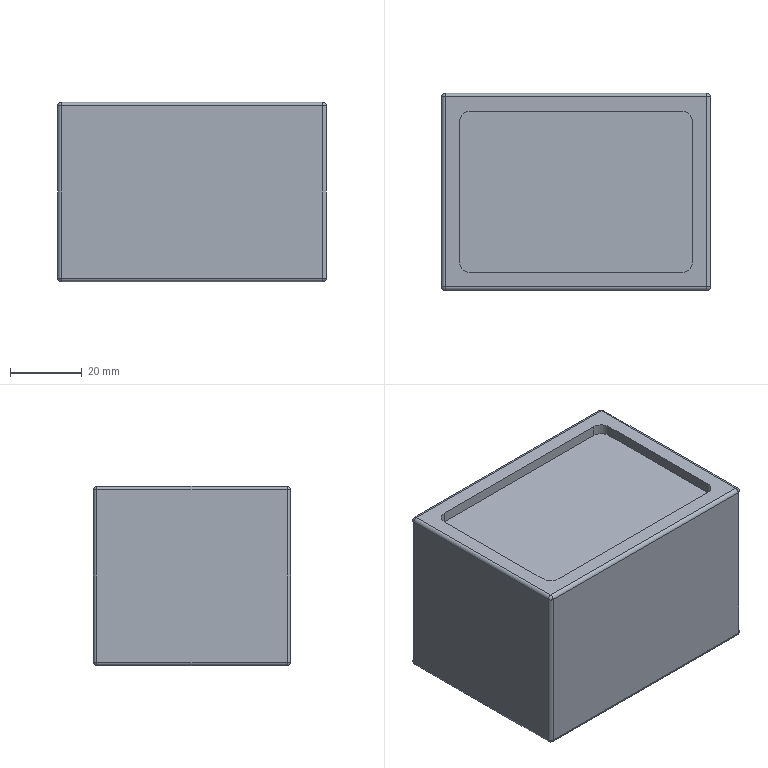Part | SolidWorks | features Fillet 2, Extrusion 1, ICE 1 | 1 solid | 35 faces | box 75 x 55 x 50 mm | volume 197345 mm3 | cylinder 16 | plane 11 | sphere 8 | commonest cylinder face diameters 2 x12 6 x4
STEP:
#1=CARTESIAN_POINT('',(0.,1.,49.));
#2=VERTEX_POINT('',#1);
#3=CARTESIAN_POINT('',(0.,54.,49.));
#4=VERTEX_POINT('',#3);
#5=CARTESIAN_POINT('',(0.,0.,49.));
#6=DIRECTION('',(0.,1.,0.));
#7=VECTOR('',#6,1000.);
#8=LINE('',#5,#7);
#9=EDGE_CURVE('',#2,#4,#8,.T.);
#10=ORIENTED_EDGE('',*,*,#9,.T.);
#11=CARTESIAN_POINT('',(0.,54.,1.));
#12=VERTEX_POINT('',#11);
#13=CARTESIAN_POINT('',(0.,54.,50.));
#14=DIRECTION('',(0.,0.,-1.));
#15=VECTOR('',#14,1000.);
#16=LINE('',#13,#15);
#17=EDGE_CURVE('',#4,#12,#16,.T.);
#18=ORIENTED_EDGE('',*,*,#17,.T.);
#19=CARTESIAN_POINT('',(0.,1.,1.));
#20=VERTEX_POINT('',#19);
#21=CARTESIAN_POINT('',(0.,0.,1.));
#22=DIRECTION('',(0.,-1.,0.));
#23=VECTOR('',#22,1000.);
#24=LINE('',#21,#23);
#25=EDGE_CURVE('',#12,#20,#24,.T.);
#26=ORIENTED_EDGE('',*,*,#25,.T.);
#27=CARTESIAN_POINT('',(0.,1.,50.));
#28=DIRECTION('',(0.,0.,1.));
#29=VECTOR('',#28,1000.);
#30=LINE('',#27,#29);
#31=EDGE_CURVE('',#20,#2,#30,.T.);
#32=ORIENTED_EDGE('',*,*,#31,.T.);
#33=EDGE_LOOP('',(#10,#18,#26,#32));
#34=FACE_OUTER_BOUND('',#33,.T.);
#35=CARTESIAN_POINT('',(0.,0.,50.));
#36=DIRECTION('',(1.,0.,0.));
#37=DIRECTION('',(0.,0.,-1.));
#38=AXIS2_PLACEMENT_3D('',#35,#36,#37);
#39=PLANE('',#38);
#40=ADVANCED_FACE('',(#34),#39,.F.);
#41=CARTESIAN_POINT('',(74.,0.,1.));
#42=VERTEX_POINT('',#41);
#43=CARTESIAN_POINT('',(74.,0.,49.));
#44=VERTEX_POINT('',#43);
#45=CARTESIAN_POINT('',(74.,0.,50.));
#46=DIRECTION('',(0.,0.,1.));
#47=VECTOR('',#46,1000.);
#48=LINE('',#45,#47);
#49=EDGE_CURVE('',#42,#44,#48,.T.);
#50=ORIENTED_EDGE('',*,*,#49,.T.);
#51=CARTESIAN_POINT('',(1.,0.,49.));
#52=VERTEX_POINT('',#51);
#53=CARTESIAN_POINT('',(0.,0.,49.));
#54=DIRECTION('',(-1.,0.,0.));
#55=VECTOR('',#54,1000.);
#56=LINE('',#53,#55);
#57=EDGE_CURVE('',#44,#52,#56,.T.);
#58=ORIENTED_EDGE('',*,*,#57,.T.);
#59=CARTESIAN_POINT('',(1.,0.,1.));
#60=VERTEX_POINT('',#59);
#61=CARTESIAN_POINT('',(1.,0.,50.));
#62=DIRECTION('',(0.,0.,-1.));
#63=VECTOR('',#62,1000.);
#64=LINE('',#61,#63);
#65=EDGE_CURVE('',#52,#60,#64,.T.);
#66=ORIENTED_EDGE('',*,*,#65,.T.);
#67=CARTESIAN_POINT('',(75.,0.,1.));
#68=DIRECTION('',(1.,0.,0.));
#69=VECTOR('',#68,1000.);
#70=LINE('',#67,#69);
#71=EDGE_CURVE('',#60,#42,#70,.T.);
#72=ORIENTED_EDGE('',*,*,#71,.T.);
#73=EDGE_LOOP('',(#50,#58,#66,#72));
#74=FACE_OUTER_BOUND('',#73,.T.);
#75=CARTESIAN_POINT('',(0.,0.,50.));
#76=DIRECTION('',(0.,1.,0.));
#77=DIRECTION('',(0.,0.,1.));
#78=AXIS2_PLACEMENT_3D('',#75,#76,#77);
#79=PLANE('',#78);
#80=ADVANCED_FACE('',(#74),#79,.F.);
#81=CARTESIAN_POINT('',(75.,54.,49.));
#82=VERTEX_POINT('',#81);
#83=CARTESIAN_POINT('',(75.,1.,49.));
#84=VERTEX_POINT('',#83);
#85=CARTESIAN_POINT('',(75.,0.,49.));
#86=DIRECTION('',(0.,-1.,0.));
#87=VECTOR('',#86,1000.);
#88=LINE('',#85,#87);
#89=EDGE_CURVE('',#82,#84,#88,.T.);
#90=ORIENTED_EDGE('',*,*,#89,.T.);
#91=CARTESIAN_POINT('',(75.,1.,1.));
#92=VERTEX_POINT('',#91);
#93=CARTESIAN_POINT('',(75.,1.,50.));
#94=DIRECTION('',(0.,0.,-1.));
#95=VECTOR('',#94,1000.);
#96=LINE('',#93,#95);
#97=EDGE_CURVE('',#84,#92,#96,.T.);
#98=ORIENTED_EDGE('',*,*,#97,.T.);
#99=CARTESIAN_POINT('',(75.,54.,1.));
#100=VERTEX_POINT('',#99);
#101=CARTESIAN_POINT('',(75.,55.,1.));
#102=DIRECTION('',(0.,1.,0.));
#103=VECTOR('',#102,1000.);
#104=LINE('',#101,#103);
#105=EDGE_CURVE('',#92,#100,#104,.T.);
#106=ORIENTED_EDGE('',*,*,#105,.T.);
#107=CARTESIAN_POINT('',(75.,54.,50.));
#108=DIRECTION('',(0.,0.,1.));
#109=VECTOR('',#108,1000.);
#110=LINE('',#107,#109);
#111=EDGE_CURVE('',#100,#82,#110,.T.);
#112=ORIENTED_EDGE('',*,*,#111,.T.);
#113=EDGE_LOOP('',(#90,#98,#106,#112));
#114=FACE_OUTER_BOUND('',#113,.T.);
#115=CARTESIAN_POINT('',(75.,0.,50.));
#116=DIRECTION('',(-1.,0.,0.));
#117=DIRECTION('',(0.,0.,1.));
#118=AXIS2_PLACEMENT_3D('',#115,#116,#117);
#119=PLANE('',#118);
#120=ADVANCED_FACE('',(#114),#119,.F.);
#121=CARTESIAN_POINT('',(1.,55.,49.));
#122=VERTEX_POINT('',#121);
#123=CARTESIAN_POINT('',(74.,55.,49.));
#124=VERTEX_POINT('',#123);
#125=CARTESIAN_POINT('',(0.,55.,49.));
#126=DIRECTION('',(1.,0.,0.));
#127=VECTOR('',#126,1000.);
#128=LINE('',#125,#127);
#129=EDGE_CURVE('',#122,#124,#128,.T.);
#130=ORIENTED_EDGE('',*,*,#129,.T.);
#131=CARTESIAN_POINT('',(74.,55.,1.));
#132=VERTEX_POINT('',#131);
#133=CARTESIAN_POINT('',(74.,55.,50.));
#134=DIRECTION('',(0.,0.,-1.));
#135=VECTOR('',#134,1000.);
#136=LINE('',#133,#135);
#137=EDGE_CURVE('',#124,#132,#136,.T.);
#138=ORIENTED_EDGE('',*,*,#137,.T.);
#139=CARTESIAN_POINT('',(1.,55.,1.));
#140=VERTEX_POINT('',#139);
#141=CARTESIAN_POINT('',(0.,55.,1.));
#142=DIRECTION('',(-1.,0.,0.));
#143=VECTOR('',#142,1000.);
#144=LINE('',#141,#143);
#145=EDGE_CURVE('',#132,#140,#144,.T.);
#146=ORIENTED_EDGE('',*,*,#145,.T.);
#147=CARTESIAN_POINT('',(1.,55.,50.));
#148=DIRECTION('',(0.,0.,1.));
#149=VECTOR('',#148,1000.);
#150=LINE('',#147,#149);
#151=EDGE_CURVE('',#140,#122,#150,.T.);
#152=ORIENTED_EDGE('',*,*,#151,.T.);
#153=EDGE_LOOP('',(#130,#138,#146,#152));
#154=FACE_OUTER_BOUND('',#153,.T.);
#155=CARTESIAN_POINT('',(0.,55.,50.));
#156=DIRECTION('',(0.,-1.,0.));
#157=DIRECTION('',(0.,0.,-1.));
#158=AXIS2_PLACEMENT_3D('',#155,#156,#157);
#159=PLANE('',#158);
#160=ADVANCED_FACE('',(#154),#159,.F.);
#161=CARTESIAN_POINT('',(1.,1.,50.));
#162=VERTEX_POINT('',#161);
#163=CARTESIAN_POINT('',(74.,1.,50.));
#164=VERTEX_POINT('',#163);
#165=CARTESIAN_POINT('',(0.,1.,50.));
#166=DIRECTION('',(1.,0.,0.));
#167=VECTOR('',#166,1000.);
#168=LINE('',#165,#167);
#169=EDGE_CURVE('',#162,#164,#168,.T.);
#170=ORIENTED_EDGE('',*,*,#169,.T.);
#171=CARTESIAN_POINT('',(74.,54.,50.));
#172=VERTEX_POINT('',#171);
#173=CARTESIAN_POINT('',(74.,0.,50.));
#174=DIRECTION('',(0.,1.,0.));
#175=VECTOR('',#174,1000.);
#176=LINE('',#173,#175);
#177=EDGE_CURVE('',#164,#172,#176,.T.);
#178=ORIENTED_EDGE('',*,*,#177,.T.);
#179=CARTESIAN_POINT('',(1.,54.,50.));
#180=VERTEX_POINT('',#179);
#181=CARTESIAN_POINT('',(0.,54.,50.));
#182=DIRECTION('',(-1.,0.,0.));
#183=VECTOR('',#182,1000.);
#184=LINE('',#181,#183);
#185=EDGE_CURVE('',#172,#180,#184,.T.);
#186=ORIENTED_EDGE('',*,*,#185,.T.);
#187=CARTESIAN_POINT('',(1.,0.,50.));
#188=DIRECTION('',(0.,-1.,0.));
#189=VECTOR('',#188,1000.);
#190=LINE('',#187,#189);
#191=EDGE_CURVE('',#180,#162,#190,.T.);
#192=ORIENTED_EDGE('',*,*,#191,.T.);
#193=EDGE_LOOP('',(#170,#178,#186,#192));
#194=FACE_OUTER_BOUND('',#193,.T.);
#195=CARTESIAN_POINT('',(8.,5.,50.));
#196=VERTEX_POINT('',#195);
#197=CARTESIAN_POINT('',(67.,5.,50.));
#198=VERTEX_POINT('',#197);
#199=CARTESIAN_POINT('',(5.,5.,50.));
#200=DIRECTION('',(1.,0.,0.));
#201=VECTOR('',#200,1000.);
#202=LINE('',#199,#201);
#203=EDGE_CURVE('',#196,#198,#202,.T.);
#204=ORIENTED_EDGE('',*,*,#203,.F.);
#205=CARTESIAN_POINT('',(5.,8.,50.));
#206=VERTEX_POINT('',#205);
#207=CARTESIAN_POINT('',(8.,8.,50.));
#208=DIRECTION('',(0.,0.,-1.));
#209=DIRECTION('',(-1.,0.,0.));
#210=AXIS2_PLACEMENT_3D('',#207,#208,#209);
#211=CIRCLE('',#210,3.);
#212=EDGE_CURVE('',#196,#206,#211,.T.);
#213=ORIENTED_EDGE('',*,*,#212,.T.);
#214=CARTESIAN_POINT('',(5.,47.,50.));
#215=VERTEX_POINT('',#214);
#216=CARTESIAN_POINT('',(5.,50.,50.));
#217=DIRECTION('',(0.,-1.,0.));
#218=VECTOR('',#217,1000.);
#219=LINE('',#216,#218);
#220=EDGE_CURVE('',#215,#206,#219,.T.);
#221=ORIENTED_EDGE('',*,*,#220,.F.);
#222=CARTESIAN_POINT('',(8.,50.,50.));
#223=VERTEX_POINT('',#222);
#224=CARTESIAN_POINT('',(8.,47.,50.));
#225=DIRECTION('',(0.,0.,-1.));
#226=DIRECTION('',(-1.,0.,0.));
#227=AXIS2_PLACEMENT_3D('',#224,#225,#226);
#228=CIRCLE('',#227,3.);
#229=EDGE_CURVE('',#215,#223,#228,.T.);
#230=ORIENTED_EDGE('',*,*,#229,.T.);
#231=CARTESIAN_POINT('',(67.,50.,50.));
#232=VERTEX_POINT('',#231);
#233=CARTESIAN_POINT('',(5.,50.,50.));
#234=DIRECTION('',(-1.,0.,0.));
#235=VECTOR('',#234,1000.);
#236=LINE('',#233,#235);
#237=EDGE_CURVE('',#232,#223,#236,.T.);
#238=ORIENTED_EDGE('',*,*,#237,.F.);
#239=CARTESIAN_POINT('',(70.,47.,50.));
#240=VERTEX_POINT('',#239);
#241=CARTESIAN_POINT('',(67.,47.,50.));
#242=DIRECTION('',(0.,0.,-1.));
#243=DIRECTION('',(-1.,0.,0.));
#244=AXIS2_PLACEMENT_3D('',#241,#242,#243);
#245=CIRCLE('',#244,3.);
#246=EDGE_CURVE('',#232,#240,#245,.T.);
#247=ORIENTED_EDGE('',*,*,#246,.T.);
#248=CARTESIAN_POINT('',(70.,8.,50.));
#249=VERTEX_POINT('',#248);
#250=CARTESIAN_POINT('',(70.,50.,50.));
#251=DIRECTION('',(0.,1.,0.));
#252=VECTOR('',#251,1000.);
#253=LINE('',#250,#252);
#254=EDGE_CURVE('',#249,#240,#253,.T.);
#255=ORIENTED_EDGE('',*,*,#254,.F.);
#256=CARTESIAN_POINT('',(67.,8.,50.));
#257=DIRECTION('',(0.,0.,-1.));
#258=DIRECTION('',(-1.,0.,0.));
#259=AXIS2_PLACEMENT_3D('',#256,#257,#258);
#260=CIRCLE('',#259,3.);
#261=EDGE_CURVE('',#249,#198,#260,.T.);
#262=ORIENTED_EDGE('',*,*,#261,.T.);
#263=EDGE_LOOP('',(#204,#213,#221,#230,#238,#247,#255,#262));
#264=FACE_BOUND('',#263,.T.);
#265=CARTESIAN_POINT('',(0.,0.,50.));
#266=DIRECTION('',(0.,0.,-1.));
#267=DIRECTION('',(-1.,0.,0.));
#268=AXIS2_PLACEMENT_3D('',#265,#266,#267);
#269=PLANE('',#268);
#270=ADVANCED_FACE('',(#194,#264),#269,.F.);
#271=CARTESIAN_POINT('',(1.,54.,0.));
#272=VERTEX_POINT('',#271);
#273=CARTESIAN_POINT('',(74.,54.,0.));
#274=VERTEX_POINT('',#273);
#275=CARTESIAN_POINT('',(75.,54.,0.));
#276=DIRECTION('',(1.,0.,0.));
#277=VECTOR('',#276,1000.);
#278=LINE('',#275,#277);
#279=EDGE_CURVE('',#272,#274,#278,.T.);
#280=ORIENTED_EDGE('',*,*,#279,.T.);
#281=CARTESIAN_POINT('',(74.,1.,0.));
#282=VERTEX_POINT('',#281);
#283=CARTESIAN_POINT('',(74.,0.,0.));
#284=DIRECTION('',(0.,-1.,0.));
#285=VECTOR('',#284,1000.);
#286=LINE('',#283,#285);
#287=EDGE_CURVE('',#274,#282,#286,.T.);
#288=ORIENTED_EDGE('',*,*,#287,.T.);
#289=CARTESIAN_POINT('',(1.,1.,0.));
#290=VERTEX_POINT('',#289);
#291=CARTESIAN_POINT('',(0.,1.,0.));
#292=DIRECTION('',(-1.,0.,0.));
#293=VECTOR('',#292,1000.);
#294=LINE('',#291,#293);
#295=EDGE_CURVE('',#282,#290,#294,.T.);
#296=ORIENTED_EDGE('',*,*,#295,.T.);
#297=CARTESIAN_POINT('',(1.,55.,0.));
#298=DIRECTION('',(0.,1.,0.));
#299=VECTOR('',#298,1000.);
#300=LINE('',#297,#299);
#301=EDGE_CURVE('',#290,#272,#300,.T.);
#302=ORIENTED_EDGE('',*,*,#301,.T.);
#303=EDGE_LOOP('',(#280,#288,#296,#302));
#304=FACE_OUTER_BOUND('',#303,.T.);
#305=CARTESIAN_POINT('',(0.,0.,0.));
#306=DIRECTION('',(0.,0.,-1.));
#307=DIRECTION('',(-1.,0.,0.));
#308=AXIS2_PLACEMENT_3D('',#305,#306,#307);
#309=PLANE('',#308);
#310=ADVANCED_FACE('',(#304),#309,.T.);
#311=ORIENTED_EDGE('',*,*,#220,.T.);
#312=CARTESIAN_POINT('',(5.,8.,47.));
#313=VERTEX_POINT('',#312);
#314=CARTESIAN_POINT('',(5.,8.,47.));
#315=DIRECTION('',(0.,0.,-1.));
#316=VECTOR('',#315,1000.);
#317=LINE('',#314,#316);
#318=EDGE_CURVE('',#206,#313,#317,.T.);
#319=ORIENTED_EDGE('',*,*,#318,.T.);
#320=CARTESIAN_POINT('',(5.,47.,47.));
#321=VERTEX_POINT('',#320);
#322=CARTESIAN_POINT('',(5.,50.,47.));
#323=DIRECTION('',(0.,-1.,0.));
#324=VECTOR('',#323,1000.);
#325=LINE('',#322,#324);
#326=EDGE_CURVE('',#321,#313,#325,.T.);
#327=ORIENTED_EDGE('',*,*,#326,.F.);
#328=CARTESIAN_POINT('',(5.,47.,50.));
#329=DIRECTION('',(0.,0.,1.));
#330=VECTOR('',#329,1000.);
#331=LINE('',#328,#330);
#332=EDGE_CURVE('',#321,#215,#331,.T.);
#333=ORIENTED_EDGE('',*,*,#332,.T.);
#334=EDGE_LOOP('',(#311,#319,#327,#333));
#335=FACE_OUTER_BOUND('',#334,.T.);
#336=CARTESIAN_POINT('',(5.,50.,47.));
#337=DIRECTION('',(-1.,0.,0.));
#338=DIRECTION('',(0.,-1.,0.));
#339=AXIS2_PLACEMENT_3D('',#336,#337,#338);
#340=PLANE('',#339);
#341=ADVANCED_FACE('',(#335),#340,.F.);
#342=CARTESIAN_POINT('',(67.,50.,47.));
#343=VERTEX_POINT('',#342);
#344=CARTESIAN_POINT('',(8.,50.,47.));
#345=VERTEX_POINT('',#344);
#346=CARTESIAN_POINT('',(5.,50.,47.));
#347=DIRECTION('',(-1.,0.,0.));
#348=VECTOR('',#347,1000.);
#349=LINE('',#346,#348);
#350=EDGE_CURVE('',#343,#345,#349,.T.);
#351=ORIENTED_EDGE('',*,*,#350,.F.);
#352=CARTESIAN_POINT('',(67.,50.,50.));
#353=DIRECTION('',(0.,0.,1.));
#354=VECTOR('',#353,1000.);
#355=LINE('',#352,#354);
#356=EDGE_CURVE('',#343,#232,#355,.T.);
#357=ORIENTED_EDGE('',*,*,#356,.T.);
#358=ORIENTED_EDGE('',*,*,#237,.T.);
#359=CARTESIAN_POINT('',(8.,50.,47.));
#360=DIRECTION('',(0.,0.,-1.));
#361=VECTOR('',#360,1000.);
#362=LINE('',#359,#361);
#363=EDGE_CURVE('',#223,#345,#362,.T.);
#364=ORIENTED_EDGE('',*,*,#363,.T.);
#365=EDGE_LOOP('',(#351,#357,#358,#364));
#366=FACE_OUTER_BOUND('',#365,.T.);
#367=CARTESIAN_POINT('',(5.,50.,47.));
#368=DIRECTION('',(0.,1.,0.));
#369=DIRECTION('',(0.,0.,1.));
#370=AXIS2_PLACEMENT_3D('',#367,#368,#369);
#371=PLANE('',#370);
#372=ADVANCED_FACE('',(#366),#371,.F.);
#373=CARTESIAN_POINT('',(70.,8.,47.));
#374=VERTEX_POINT('',#373);
#375=CARTESIAN_POINT('',(70.,47.,47.));
#376=VERTEX_POINT('',#375);
#377=CARTESIAN_POINT('',(70.,50.,47.));
#378=DIRECTION('',(0.,1.,0.));
#379=VECTOR('',#378,1000.);
#380=LINE('',#377,#379);
#381=EDGE_CURVE('',#374,#376,#380,.T.);
#382=ORIENTED_EDGE('',*,*,#381,.F.);
#383=CARTESIAN_POINT('',(70.,8.,50.));
#384=DIRECTION('',(0.,0.,1.));
#385=VECTOR('',#384,1000.);
#386=LINE('',#383,#385);
#387=EDGE_CURVE('',#374,#249,#386,.T.);
#388=ORIENTED_EDGE('',*,*,#387,.T.);
#389=ORIENTED_EDGE('',*,*,#254,.T.);
#390=CARTESIAN_POINT('',(70.,47.,47.));
#391=DIRECTION('',(0.,0.,-1.));
#392=VECTOR('',#391,1000.);
#393=LINE('',#390,#392);
#394=EDGE_CURVE('',#240,#376,#393,.T.);
#395=ORIENTED_EDGE('',*,*,#394,.T.);
#396=EDGE_LOOP('',(#382,#388,#389,#395));
#397=FACE_OUTER_BOUND('',#396,.T.);
#398=CARTESIAN_POINT('',(70.,50.,47.));
#399=DIRECTION('',(1.,0.,0.));
#400=DIRECTION('',(0.,0.,-1.));
#401=AXIS2_PLACEMENT_3D('',#398,#399,#400);
#402=PLANE('',#401);
#403=ADVANCED_FACE('',(#397),#402,.F.);
#404=CARTESIAN_POINT('',(8.,5.,47.));
#405=VERTEX_POINT('',#404);
#406=CARTESIAN_POINT('',(67.,5.,47.));
#407=VERTEX_POINT('',#406);
#408=CARTESIAN_POINT('',(5.,5.,47.));
#409=DIRECTION('',(1.,0.,0.));
#410=VECTOR('',#409,1000.);
#411=LINE('',#408,#410);
#412=EDGE_CURVE('',#405,#407,#411,.T.);
#413=ORIENTED_EDGE('',*,*,#412,.F.);
#414=CARTESIAN_POINT('',(8.,5.,50.));
#415=DIRECTION('',(0.,0.,1.));
#416=VECTOR('',#415,1000.);
#417=LINE('',#414,#416);
#418=EDGE_CURVE('',#405,#196,#417,.T.);
#419=ORIENTED_EDGE('',*,*,#418,.T.);
#420=ORIENTED_EDGE('',*,*,#203,.T.);
#421=CARTESIAN_POINT('',(67.,5.,47.));
#422=DIRECTION('',(0.,0.,-1.));
#423=VECTOR('',#422,1000.);
#424=LINE('',#421,#423);
#425=EDGE_CURVE('',#198,#407,#424,.T.);
#426=ORIENTED_EDGE('',*,*,#425,.T.);
#427=EDGE_LOOP('',(#413,#419,#420,#426));
#428=FACE_OUTER_BOUND('',#427,.T.);
#429=CARTESIAN_POINT('',(5.,5.,47.));
#430=DIRECTION('',(0.,-1.,0.));
#431=DIRECTION('',(0.,0.,-1.));
#432=AXIS2_PLACEMENT_3D('',#429,#430,#431);
#433=PLANE('',#432);
#434=ADVANCED_FACE('',(#428),#433,.F.);
#435=ORIENTED_EDGE('',*,*,#326,.T.);
#436=CARTESIAN_POINT('',(8.,8.,47.));
#437=DIRECTION('',(0.,0.,1.));
#438=DIRECTION('',(1.,0.,0.));
#439=AXIS2_PLACEMENT_3D('',#436,#437,#438);
#440=CIRCLE('',#439,3.);
#441=EDGE_CURVE('',#313,#405,#440,.T.);
#442=ORIENTED_EDGE('',*,*,#441,.T.);
#443=ORIENTED_EDGE('',*,*,#412,.T.);
#444=CARTESIAN_POINT('',(67.,8.,47.));
#445=DIRECTION('',(0.,0.,1.));
#446=DIRECTION('',(1.,0.,0.));
#447=AXIS2_PLACEMENT_3D('',#444,#445,#446);
#448=CIRCLE('',#447,3.);
#449=EDGE_CURVE('',#407,#374,#448,.T.);
#450=ORIENTED_EDGE('',*,*,#449,.T.);
#451=ORIENTED_EDGE('',*,*,#381,.T.);
#452=CARTESIAN_POINT('',(67.,47.,47.));
#453=DIRECTION('',(0.,0.,1.));
#454=DIRECTION('',(1.,0.,0.));
#455=AXIS2_PLACEMENT_3D('',#452,#453,#454);
#456=CIRCLE('',#455,3.);
#457=EDGE_CURVE('',#376,#343,#456,.T.);
#458=ORIENTED_EDGE('',*,*,#457,.T.);
#459=ORIENTED_EDGE('',*,*,#350,.T.);
#460=CARTESIAN_POINT('',(8.,47.,47.));
#461=DIRECTION('',(0.,0.,1.));
#462=DIRECTION('',(1.,0.,0.));
#463=AXIS2_PLACEMENT_3D('',#460,#461,#462);
#464=CIRCLE('',#463,3.);
#465=EDGE_CURVE('',#345,#321,#464,.T.);
#466=ORIENTED_EDGE('',*,*,#465,.T.);
#467=EDGE_LOOP('',(#435,#442,#443,#450,#451,#458,#459,#466));
#468=FACE_OUTER_BOUND('',#467,.T.);
#469=CARTESIAN_POINT('',(0.,0.,47.));
#470=DIRECTION('',(0.,0.,1.));
#471=DIRECTION('',(1.,0.,0.));
#472=AXIS2_PLACEMENT_3D('',#469,#470,#471);
#473=PLANE('',#472);
#474=ADVANCED_FACE('',(#468),#473,.T.);
#475=ORIENTED_EDGE('',*,*,#441,.F.);
#476=ORIENTED_EDGE('',*,*,#318,.F.);
#477=ORIENTED_EDGE('',*,*,#212,.F.);
#478=ORIENTED_EDGE('',*,*,#418,.F.);
#479=EDGE_LOOP('',(#475,#476,#477,#478));
#480=FACE_OUTER_BOUND('',#479,.T.);
#481=CARTESIAN_POINT('',(8.,8.,47.));
#482=DIRECTION('',(0.,0.,-1.));
#483=DIRECTION('',(-1.,0.,0.));
#484=AXIS2_PLACEMENT_3D('',#481,#482,#483);
#485=CYLINDRICAL_SURFACE('',#484,3.);
#486=ADVANCED_FACE('',(#480),#485,.F.);
#487=ORIENTED_EDGE('',*,*,#449,.F.);
#488=ORIENTED_EDGE('',*,*,#425,.F.);
#489=ORIENTED_EDGE('',*,*,#261,.F.);
#490=ORIENTED_EDGE('',*,*,#387,.F.);
#491=EDGE_LOOP('',(#487,#488,#489,#490));
#492=FACE_OUTER_BOUND('',#491,.T.);
#493=CARTESIAN_POINT('',(67.,8.,47.));
#494=DIRECTION('',(0.,0.,-1.));
#495=DIRECTION('',(-1.,0.,0.));
#496=AXIS2_PLACEMENT_3D('',#493,#494,#495);
#497=CYLINDRICAL_SURFACE('',#496,3.);
#498=ADVANCED_FACE('',(#492),#497,.F.);
#499=ORIENTED_EDGE('',*,*,#457,.F.);
#500=ORIENTED_EDGE('',*,*,#394,.F.);
#501=ORIENTED_EDGE('',*,*,#246,.F.);
#502=ORIENTED_EDGE('',*,*,#356,.F.);
#503=EDGE_LOOP('',(#499,#500,#501,#502));
#504=FACE_OUTER_BOUND('',#503,.T.);
#505=CARTESIAN_POINT('',(67.,47.,47.));
#506=DIRECTION('',(0.,0.,-1.));
#507=DIRECTION('',(-1.,0.,0.));
#508=AXIS2_PLACEMENT_3D('',#505,#506,#507);
#509=CYLINDRICAL_SURFACE('',#508,3.);
#510=ADVANCED_FACE('',(#504),#509,.F.);
#511=ORIENTED_EDGE('',*,*,#465,.F.);
#512=ORIENTED_EDGE('',*,*,#363,.F.);
#513=ORIENTED_EDGE('',*,*,#229,.F.);
#514=ORIENTED_EDGE('',*,*,#332,.F.);
#515=EDGE_LOOP('',(#511,#512,#513,#514));
#516=FACE_OUTER_BOUND('',#515,.T.);
#517=CARTESIAN_POINT('',(8.,47.,47.));
#518=DIRECTION('',(0.,0.,-1.));
#519=DIRECTION('',(-1.,0.,0.));
#520=AXIS2_PLACEMENT_3D('',#517,#518,#519);
#521=CYLINDRICAL_SURFACE('',#520,3.);
#522=ADVANCED_FACE('',(#516),#521,.F.);
#523=CARTESIAN_POINT('',(1.,1.,1.));
#524=DIRECTION('',(0.,-1.,0.));
#525=DIRECTION('',(0.,0.,-1.));
#526=AXIS2_PLACEMENT_3D('',#523,#524,#525);
#527=CIRCLE('',#526,1.);
#528=EDGE_CURVE('',#20,#290,#527,.T.);
#529=ORIENTED_EDGE('',*,*,#528,.F.);
#530=ORIENTED_EDGE('',*,*,#25,.F.);
#531=CARTESIAN_POINT('',(1.,54.,1.));
#532=DIRECTION('',(0.,1.,0.));
#533=DIRECTION('',(0.,0.,1.));
#534=AXIS2_PLACEMENT_3D('',#531,#532,#533);
#535=CIRCLE('',#534,1.);
#536=EDGE_CURVE('',#272,#12,#535,.T.);
#537=ORIENTED_EDGE('',*,*,#536,.F.);
#538=ORIENTED_EDGE('',*,*,#301,.F.);
#539=EDGE_LOOP('',(#529,#530,#537,#538));
#540=FACE_OUTER_BOUND('',#539,.T.);
#541=CARTESIAN_POINT('',(1.,0.,1.));
#542=DIRECTION('',(0.,1.,0.));
#543=DIRECTION('',(0.,0.,1.));
#544=AXIS2_PLACEMENT_3D('',#541,#542,#543);
#545=CYLINDRICAL_SURFACE('',#544,1.);
#546=ADVANCED_FACE('',(#540),#545,.T.);
#547=CARTESIAN_POINT('',(1.,1.,1.));
#548=DIRECTION('',(0.,0.,1.));
#549=DIRECTION('',(-1.,0.,0.));
#550=AXIS2_PLACEMENT_3D('',#547,#548,#549);
#551=CIRCLE('',#550,1.);
#552=EDGE_CURVE('',#20,#60,#551,.T.);
#553=ORIENTED_EDGE('',*,*,#552,.F.);
#554=ORIENTED_EDGE('',*,*,#528,.T.);
#555=CARTESIAN_POINT('',(1.,1.,1.));
#556=DIRECTION('',(1.,0.,0.));
#557=DIRECTION('',(0.,0.,1.));
#558=AXIS2_PLACEMENT_3D('',#555,#556,#557);
#559=CIRCLE('',#558,1.);
#560=EDGE_CURVE('',#60,#290,#559,.T.);
#561=ORIENTED_EDGE('',*,*,#560,.F.);
#562=EDGE_LOOP('',(#553,#554,#561));
#563=FACE_OUTER_BOUND('',#562,.T.);
#564=CARTESIAN_POINT('',(1.,1.,1.));
#565=DIRECTION('',(0.,1.,0.));
#566=DIRECTION('',(1.,0.,0.));
#567=AXIS2_PLACEMENT_3D('',#564,#565,#566);
#568=SPHERICAL_SURFACE('',#567,1.);
#569=ADVANCED_FACE('',(#563),#568,.T.);
#570=CARTESIAN_POINT('',(1.,54.,1.));
#571=DIRECTION('',(1.,0.,0.));
#572=DIRECTION('',(0.,0.,1.));
#573=AXIS2_PLACEMENT_3D('',#570,#571,#572);
#574=CIRCLE('',#573,1.);
#575=EDGE_CURVE('',#272,#140,#574,.T.);
#576=ORIENTED_EDGE('',*,*,#575,.F.);
#577=ORIENTED_EDGE('',*,*,#536,.T.);
#578=CARTESIAN_POINT('',(1.,54.,1.));
#579=DIRECTION('',(0.,0.,1.));
#580=DIRECTION('',(-1.,0.,0.));
#581=AXIS2_PLACEMENT_3D('',#578,#579,#580);
#582=CIRCLE('',#581,1.);
#583=EDGE_CURVE('',#140,#12,#582,.T.);
#584=ORIENTED_EDGE('',*,*,#583,.F.);
#585=EDGE_LOOP('',(#576,#577,#584));
#586=FACE_OUTER_BOUND('',#585,.T.);
#587=CARTESIAN_POINT('',(1.,54.,1.));
#588=DIRECTION('',(0.,1.,0.));
#589=DIRECTION('',(1.,0.,0.));
#590=AXIS2_PLACEMENT_3D('',#587,#588,#589);
#591=SPHERICAL_SURFACE('',#590,1.);
#592=ADVANCED_FACE('',(#586),#591,.T.);
#593=ORIENTED_EDGE('',*,*,#560,.T.);
#594=ORIENTED_EDGE('',*,*,#295,.F.);
#595=CARTESIAN_POINT('',(74.,1.,1.));
#596=DIRECTION('',(1.,0.,0.));
#597=DIRECTION('',(0.,0.,-1.));
#598=AXIS2_PLACEMENT_3D('',#595,#596,#597);
#599=CIRCLE('',#598,1.);
#600=EDGE_CURVE('',#42,#282,#599,.T.);
#601=ORIENTED_EDGE('',*,*,#600,.F.);
#602=ORIENTED_EDGE('',*,*,#71,.F.);
#603=EDGE_LOOP('',(#593,#594,#601,#602));
#604=FACE_OUTER_BOUND('',#603,.T.);
#605=CARTESIAN_POINT('',(0.,1.,1.));
#606=DIRECTION('',(-1.,0.,0.));
#607=DIRECTION('',(0.,0.,1.));
#608=AXIS2_PLACEMENT_3D('',#605,#606,#607);
#609=CYLINDRICAL_SURFACE('',#608,1.);
#610=ADVANCED_FACE('',(#604),#609,.T.);
#611=ORIENTED_EDGE('',*,*,#552,.T.);
#612=ORIENTED_EDGE('',*,*,#65,.F.);
#613=CARTESIAN_POINT('',(1.,1.,49.));
#614=DIRECTION('',(0.,0.,1.));
#615=DIRECTION('',(1.,0.,0.));
#616=AXIS2_PLACEMENT_3D('',#613,#614,#615);
#617=CIRCLE('',#616,1.);
#618=EDGE_CURVE('',#2,#52,#617,.T.);
#619=ORIENTED_EDGE('',*,*,#618,.F.);
#620=ORIENTED_EDGE('',*,*,#31,.F.);
#621=EDGE_LOOP('',(#611,#612,#619,#620));
#622=FACE_OUTER_BOUND('',#621,.T.);
#623=CARTESIAN_POINT('',(1.,1.,50.));
#624=DIRECTION('',(0.,0.,-1.));
#625=DIRECTION('',(-1.,0.,0.));
#626=AXIS2_PLACEMENT_3D('',#623,#624,#625);
#627=CYLINDRICAL_SURFACE('',#626,1.);
#628=ADVANCED_FACE('',(#622),#627,.T.);
#629=CARTESIAN_POINT('',(1.,54.,49.));
#630=DIRECTION('',(0.,1.,0.));
#631=DIRECTION('',(0.,0.,1.));
#632=AXIS2_PLACEMENT_3D('',#629,#630,#631);
#633=CIRCLE('',#632,1.);
#634=EDGE_CURVE('',#4,#180,#633,.T.);
#635=ORIENTED_EDGE('',*,*,#634,.F.);
#636=ORIENTED_EDGE('',*,*,#9,.F.);
#637=CARTESIAN_POINT('',(1.,1.,49.));
#638=DIRECTION('',(0.,-1.,0.));
#639=DIRECTION('',(0.,0.,-1.));
#640=AXIS2_PLACEMENT_3D('',#637,#638,#639);
#641=CIRCLE('',#640,1.);
#642=EDGE_CURVE('',#162,#2,#641,.T.);
#643=ORIENTED_EDGE('',*,*,#642,.F.);
#644=ORIENTED_EDGE('',*,*,#191,.F.);
#645=EDGE_LOOP('',(#635,#636,#643,#644));
#646=FACE_OUTER_BOUND('',#645,.T.);
#647=CARTESIAN_POINT('',(1.,0.,49.));
#648=DIRECTION('',(0.,-1.,0.));
#649=DIRECTION('',(0.,0.,-1.));
#650=AXIS2_PLACEMENT_3D('',#647,#648,#649);
#651=CYLINDRICAL_SURFACE('',#650,1.);
#652=ADVANCED_FACE('',(#646),#651,.T.);
#653=ORIENTED_EDGE('',*,*,#583,.T.);
#654=ORIENTED_EDGE('',*,*,#17,.F.);
#655=CARTESIAN_POINT('',(1.,54.,49.));
#656=DIRECTION('',(0.,0.,1.));
#657=DIRECTION('',(1.,0.,0.));
#658=AXIS2_PLACEMENT_3D('',#655,#656,#657);
#659=CIRCLE('',#658,1.);
#660=EDGE_CURVE('',#122,#4,#659,.T.);
#661=ORIENTED_EDGE('',*,*,#660,.F.);
#662=ORIENTED_EDGE('',*,*,#151,.F.);
#663=EDGE_LOOP('',(#653,#654,#661,#662));
#664=FACE_OUTER_BOUND('',#663,.T.);
#665=CARTESIAN_POINT('',(1.,54.,50.));
#666=DIRECTION('',(0.,0.,-1.));
#667=DIRECTION('',(-1.,0.,0.));
#668=AXIS2_PLACEMENT_3D('',#665,#666,#667);
#669=CYLINDRICAL_SURFACE('',#668,1.);
#670=ADVANCED_FACE('',(#664),#669,.T.);
#671=ORIENTED_EDGE('',*,*,#575,.T.);
#672=ORIENTED_EDGE('',*,*,#145,.F.);
#673=CARTESIAN_POINT('',(74.,54.,1.));
#674=DIRECTION('',(1.,0.,0.));
#675=DIRECTION('',(0.,0.,-1.));
#676=AXIS2_PLACEMENT_3D('',#673,#674,#675);
#677=CIRCLE('',#676,1.);
#678=EDGE_CURVE('',#274,#132,#677,.T.);
#679=ORIENTED_EDGE('',*,*,#678,.F.);
#680=ORIENTED_EDGE('',*,*,#279,.F.);
#681=EDGE_LOOP('',(#671,#672,#679,#680));
#682=FACE_OUTER_BOUND('',#681,.T.);
#683=CARTESIAN_POINT('',(0.,54.,1.));
#684=DIRECTION('',(1.,0.,0.));
#685=DIRECTION('',(0.,0.,-1.));
#686=AXIS2_PLACEMENT_3D('',#683,#684,#685);
#687=CYLINDRICAL_SURFACE('',#686,1.);
#688=ADVANCED_FACE('',(#682),#687,.T.);
#689=CARTESIAN_POINT('',(74.,1.,1.));
#690=DIRECTION('',(0.,-1.,0.));
#691=DIRECTION('',(0.,0.,-1.));
#692=AXIS2_PLACEMENT_3D('',#689,#690,#691);
#693=CIRCLE('',#692,1.);
#694=EDGE_CURVE('',#282,#92,#693,.T.);
#695=ORIENTED_EDGE('',*,*,#694,.F.);
#696=ORIENTED_EDGE('',*,*,#287,.F.);
#697=CARTESIAN_POINT('',(74.,54.,1.));
#698=DIRECTION('',(0.,1.,0.));
#699=DIRECTION('',(0.,0.,1.));
#700=AXIS2_PLACEMENT_3D('',#697,#698,#699);
#701=CIRCLE('',#700,1.);
#702=EDGE_CURVE('',#100,#274,#701,.T.);
#703=ORIENTED_EDGE('',*,*,#702,.F.);
#704=ORIENTED_EDGE('',*,*,#105,.F.);
#705=EDGE_LOOP('',(#695,#696,#703,#704));
#706=FACE_OUTER_BOUND('',#705,.T.);
#707=CARTESIAN_POINT('',(74.,0.,1.));
#708=DIRECTION('',(0.,-1.,0.));
#709=DIRECTION('',(0.,0.,-1.));
#710=AXIS2_PLACEMENT_3D('',#707,#708,#709);
#711=CYLINDRICAL_SURFACE('',#710,1.);
#712=ADVANCED_FACE('',(#706),#711,.T.);
#713=ORIENTED_EDGE('',*,*,#600,.T.);
#714=ORIENTED_EDGE('',*,*,#694,.T.);
#715=CARTESIAN_POINT('',(74.,1.,1.));
#716=DIRECTION('',(0.,0.,1.));
#717=DIRECTION('',(-1.,0.,0.));
#718=AXIS2_PLACEMENT_3D('',#715,#716,#717);
#719=CIRCLE('',#718,1.);
#720=EDGE_CURVE('',#42,#92,#719,.T.);
#721=ORIENTED_EDGE('',*,*,#720,.F.);
#722=EDGE_LOOP('',(#713,#714,#721));
#723=FACE_OUTER_BOUND('',#722,.T.);
#724=CARTESIAN_POINT('',(74.,1.,1.));
#725=DIRECTION('',(0.,1.,0.));
#726=DIRECTION('',(1.,0.,0.));
#727=AXIS2_PLACEMENT_3D('',#724,#725,#726);
#728=SPHERICAL_SURFACE('',#727,1.);
#729=ADVANCED_FACE('',(#723),#728,.T.);
#730=ORIENTED_EDGE('',*,*,#642,.T.);
#731=ORIENTED_EDGE('',*,*,#618,.T.);
#732=CARTESIAN_POINT('',(1.,1.,49.));
#733=DIRECTION('',(1.,0.,0.));
#734=DIRECTION('',(0.,0.,1.));
#735=AXIS2_PLACEMENT_3D('',#732,#733,#734);
#736=CIRCLE('',#735,1.);
#737=EDGE_CURVE('',#162,#52,#736,.T.);
#738=ORIENTED_EDGE('',*,*,#737,.F.);
#739=EDGE_LOOP('',(#730,#731,#738));
#740=FACE_OUTER_BOUND('',#739,.T.);
#741=CARTESIAN_POINT('',(1.,1.,49.));
#742=DIRECTION('',(0.,1.,0.));
#743=DIRECTION('',(1.,0.,0.));
#744=AXIS2_PLACEMENT_3D('',#741,#742,#743);
#745=SPHERICAL_SURFACE('',#744,1.);
#746=ADVANCED_FACE('',(#740),#745,.T.);
#747=ORIENTED_EDGE('',*,*,#660,.T.);
#748=ORIENTED_EDGE('',*,*,#634,.T.);
#749=CARTESIAN_POINT('',(1.,54.,49.));
#750=DIRECTION('',(1.,0.,0.));
#751=DIRECTION('',(0.,0.,1.));
#752=AXIS2_PLACEMENT_3D('',#749,#750,#751);
#753=CIRCLE('',#752,1.);
#754=EDGE_CURVE('',#122,#180,#753,.T.);
#755=ORIENTED_EDGE('',*,*,#754,.F.);
#756=EDGE_LOOP('',(#747,#748,#755));
#757=FACE_OUTER_BOUND('',#756,.T.);
#758=CARTESIAN_POINT('',(1.,54.,49.));
#759=DIRECTION('',(0.,1.,0.));
#760=DIRECTION('',(1.,0.,0.));
#761=AXIS2_PLACEMENT_3D('',#758,#759,#760);
#762=SPHERICAL_SURFACE('',#761,1.);
#763=ADVANCED_FACE('',(#757),#762,.T.);
#764=ORIENTED_EDGE('',*,*,#702,.T.);
#765=ORIENTED_EDGE('',*,*,#678,.T.);
#766=CARTESIAN_POINT('',(74.,54.,1.));
#767=DIRECTION('',(0.,0.,1.));
#768=DIRECTION('',(-1.,0.,0.));
#769=AXIS2_PLACEMENT_3D('',#766,#767,#768);
#770=CIRCLE('',#769,1.);
#771=EDGE_CURVE('',#100,#132,#770,.T.);
#772=ORIENTED_EDGE('',*,*,#771,.F.);
#773=EDGE_LOOP('',(#764,#765,#772));
#774=FACE_OUTER_BOUND('',#773,.T.);
#775=CARTESIAN_POINT('',(74.,54.,1.));
#776=DIRECTION('',(0.,1.,0.));
#777=DIRECTION('',(1.,0.,0.));
#778=AXIS2_PLACEMENT_3D('',#775,#776,#777);
#779=SPHERICAL_SURFACE('',#778,1.);
#780=ADVANCED_FACE('',(#774),#779,.T.);
#781=ORIENTED_EDGE('',*,*,#720,.T.);
#782=ORIENTED_EDGE('',*,*,#97,.F.);
#783=CARTESIAN_POINT('',(74.,1.,49.));
#784=DIRECTION('',(0.,0.,1.));
#785=DIRECTION('',(1.,0.,0.));
#786=AXIS2_PLACEMENT_3D('',#783,#784,#785);
#787=CIRCLE('',#786,1.);
#788=EDGE_CURVE('',#44,#84,#787,.T.);
#789=ORIENTED_EDGE('',*,*,#788,.F.);
#790=ORIENTED_EDGE('',*,*,#49,.F.);
#791=EDGE_LOOP('',(#781,#782,#789,#790));
#792=FACE_OUTER_BOUND('',#791,.T.);
#793=CARTESIAN_POINT('',(74.,1.,50.));
#794=DIRECTION('',(0.,0.,-1.));
#795=DIRECTION('',(-1.,0.,0.));
#796=AXIS2_PLACEMENT_3D('',#793,#794,#795);
#797=CYLINDRICAL_SURFACE('',#796,1.);
#798=ADVANCED_FACE('',(#792),#797,.T.);
#799=ORIENTED_EDGE('',*,*,#737,.T.);
#800=ORIENTED_EDGE('',*,*,#57,.F.);
#801=CARTESIAN_POINT('',(74.,1.,49.));
#802=DIRECTION('',(1.,0.,0.));
#803=DIRECTION('',(0.,0.,-1.));
#804=AXIS2_PLACEMENT_3D('',#801,#802,#803);
#805=CIRCLE('',#804,1.);
#806=EDGE_CURVE('',#164,#44,#805,.T.);
#807=ORIENTED_EDGE('',*,*,#806,.F.);
#808=ORIENTED_EDGE('',*,*,#169,.F.);
#809=EDGE_LOOP('',(#799,#800,#807,#808));
#810=FACE_OUTER_BOUND('',#809,.T.);
#811=CARTESIAN_POINT('',(0.,1.,49.));
#812=DIRECTION('',(1.,0.,0.));
#813=DIRECTION('',(0.,0.,-1.));
#814=AXIS2_PLACEMENT_3D('',#811,#812,#813);
#815=CYLINDRICAL_SURFACE('',#814,1.);
#816=ADVANCED_FACE('',(#810),#815,.T.);
#817=ORIENTED_EDGE('',*,*,#754,.T.);
#818=ORIENTED_EDGE('',*,*,#185,.F.);
#819=CARTESIAN_POINT('',(74.,54.,49.));
#820=DIRECTION('',(1.,0.,0.));
#821=DIRECTION('',(0.,0.,-1.));
#822=AXIS2_PLACEMENT_3D('',#819,#820,#821);
#823=CIRCLE('',#822,1.);
#824=EDGE_CURVE('',#124,#172,#823,.T.);
#825=ORIENTED_EDGE('',*,*,#824,.F.);
#826=ORIENTED_EDGE('',*,*,#129,.F.);
#827=EDGE_LOOP('',(#817,#818,#825,#826));
#828=FACE_OUTER_BOUND('',#827,.T.);
#829=CARTESIAN_POINT('',(0.,54.,49.));
#830=DIRECTION('',(-1.,0.,0.));
#831=DIRECTION('',(0.,0.,1.));
#832=AXIS2_PLACEMENT_3D('',#829,#830,#831);
#833=CYLINDRICAL_SURFACE('',#832,1.);
#834=ADVANCED_FACE('',(#828),#833,.T.);
#835=ORIENTED_EDGE('',*,*,#771,.T.);
#836=ORIENTED_EDGE('',*,*,#137,.F.);
#837=CARTESIAN_POINT('',(74.,54.,49.));
#838=DIRECTION('',(0.,0.,1.));
#839=DIRECTION('',(1.,0.,0.));
#840=AXIS2_PLACEMENT_3D('',#837,#838,#839);
#841=CIRCLE('',#840,1.);
#842=EDGE_CURVE('',#82,#124,#841,.T.);
#843=ORIENTED_EDGE('',*,*,#842,.F.);
#844=ORIENTED_EDGE('',*,*,#111,.F.);
#845=EDGE_LOOP('',(#835,#836,#843,#844));
#846=FACE_OUTER_BOUND('',#845,.T.);
#847=CARTESIAN_POINT('',(74.,54.,50.));
#848=DIRECTION('',(0.,0.,-1.));
#849=DIRECTION('',(-1.,0.,0.));
#850=AXIS2_PLACEMENT_3D('',#847,#848,#849);
#851=CYLINDRICAL_SURFACE('',#850,1.);
#852=ADVANCED_FACE('',(#846),#851,.T.);
#853=ORIENTED_EDGE('',*,*,#806,.T.);
#854=ORIENTED_EDGE('',*,*,#788,.T.);
#855=CARTESIAN_POINT('',(74.,1.,49.));
#856=DIRECTION('',(0.,1.,0.));
#857=DIRECTION('',(0.,0.,-1.));
#858=AXIS2_PLACEMENT_3D('',#855,#856,#857);
#859=CIRCLE('',#858,1.);
#860=EDGE_CURVE('',#164,#84,#859,.T.);
#861=ORIENTED_EDGE('',*,*,#860,.F.);
#862=EDGE_LOOP('',(#853,#854,#861));
#863=FACE_OUTER_BOUND('',#862,.T.);
#864=CARTESIAN_POINT('',(74.,1.,49.));
#865=DIRECTION('',(0.,1.,0.));
#866=DIRECTION('',(1.,0.,0.));
#867=AXIS2_PLACEMENT_3D('',#864,#865,#866);
#868=SPHERICAL_SURFACE('',#867,1.);
#869=ADVANCED_FACE('',(#863),#868,.T.);
#870=ORIENTED_EDGE('',*,*,#842,.T.);
#871=ORIENTED_EDGE('',*,*,#824,.T.);
#872=CARTESIAN_POINT('',(74.,54.,49.));
#873=DIRECTION('',(0.,-1.,0.));
#874=DIRECTION('',(0.,0.,1.));
#875=AXIS2_PLACEMENT_3D('',#872,#873,#874);
#876=CIRCLE('',#875,1.);
#877=EDGE_CURVE('',#82,#172,#876,.T.);
#878=ORIENTED_EDGE('',*,*,#877,.F.);
#879=EDGE_LOOP('',(#870,#871,#878));
#880=FACE_OUTER_BOUND('',#879,.T.);
#881=CARTESIAN_POINT('',(74.,54.,49.));
#882=DIRECTION('',(0.,1.,0.));
#883=DIRECTION('',(1.,0.,0.));
#884=AXIS2_PLACEMENT_3D('',#881,#882,#883);
#885=SPHERICAL_SURFACE('',#884,1.);
#886=ADVANCED_FACE('',(#880),#885,.T.);
#887=ORIENTED_EDGE('',*,*,#860,.T.);
#888=ORIENTED_EDGE('',*,*,#89,.F.);
#889=ORIENTED_EDGE('',*,*,#877,.T.);
#890=ORIENTED_EDGE('',*,*,#177,.F.);
#891=EDGE_LOOP('',(#887,#888,#889,#890));
#892=FACE_OUTER_BOUND('',#891,.T.);
#893=CARTESIAN_POINT('',(74.,0.,49.));
#894=DIRECTION('',(0.,1.,0.));
#895=DIRECTION('',(0.,0.,1.));
#896=AXIS2_PLACEMENT_3D('',#893,#894,#895);
#897=CYLINDRICAL_SURFACE('',#896,1.);
#898=ADVANCED_FACE('',(#892),#897,.T.);
#899=CLOSED_SHELL('',(#40,#80,#120,#160,#270,#310,#341,#372,#403,#434,#474,#486,#498,#510,#522,#546,#569,#592,#610,#628,#652,#670,#688,#712,#729,#746,#763,#780,#798,#816,#834,#852,#869,#886,#898));
#900=MANIFOLD_SOLID_BREP('',#899);
#901=CARTESIAN_POINT('',(0.,0.,0.));
#902=DIRECTION('',(0.,0.,1.));
#903=DIRECTION('',(1.,0.,0.));
#904=AXIS2_PLACEMENT_3D('',#901,#902,#903);
#905=(LENGTH_UNIT()NAMED_UNIT(*)SI_UNIT(.MILLI.,.METRE.));
#906=UNCERTAINTY_MEASURE_WITH_UNIT(LENGTH_MEASURE(0.00001),#905,'','');
#907=(NAMED_UNIT(*)PLANE_ANGLE_UNIT()SI_UNIT($,.RADIAN.));
#908=(NAMED_UNIT(*)SI_UNIT($,.STERADIAN.)SOLID_ANGLE_UNIT());
#909=(GEOMETRIC_REPRESENTATION_CONTEXT(3)GLOBAL_UNCERTAINTY_ASSIGNED_CONTEXT((#906))GLOBAL_UNIT_ASSIGNED_CONTEXT((#905,#907,#908))REPRESENTATION_CONTEXT('',''));
#910=ADVANCED_BREP_SHAPE_REPRESENTATION('',(#900,#904),#909);